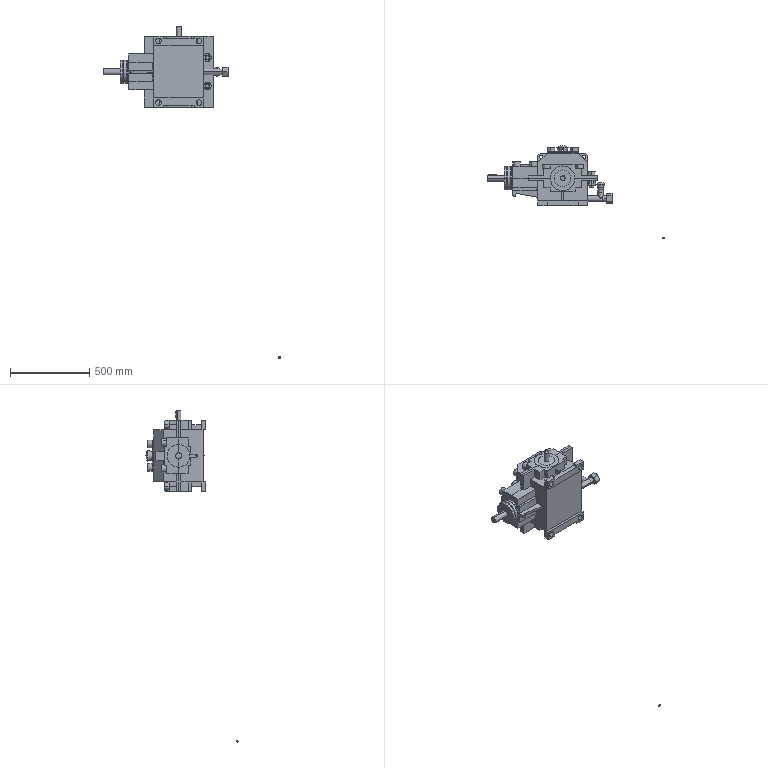Part | SolidWorks | features BaseBody 37, Scale 1 | 38 solids | 2064 faces | box 1119 x 581.368 x 2095 mm | volume 29257315 mm3 | plane 553 | sphere 456 | cylinder 357 | cone 303 | torus 276 | spline 119 | commonest cylinder face diameters 27 x64 30 x46 45 x29 48 x28 36 x16 24 x14